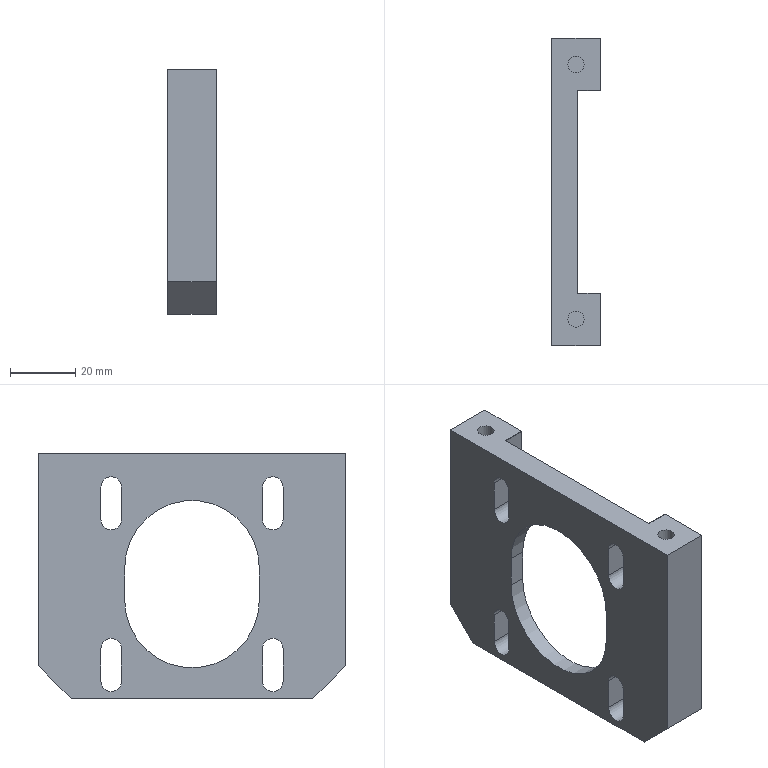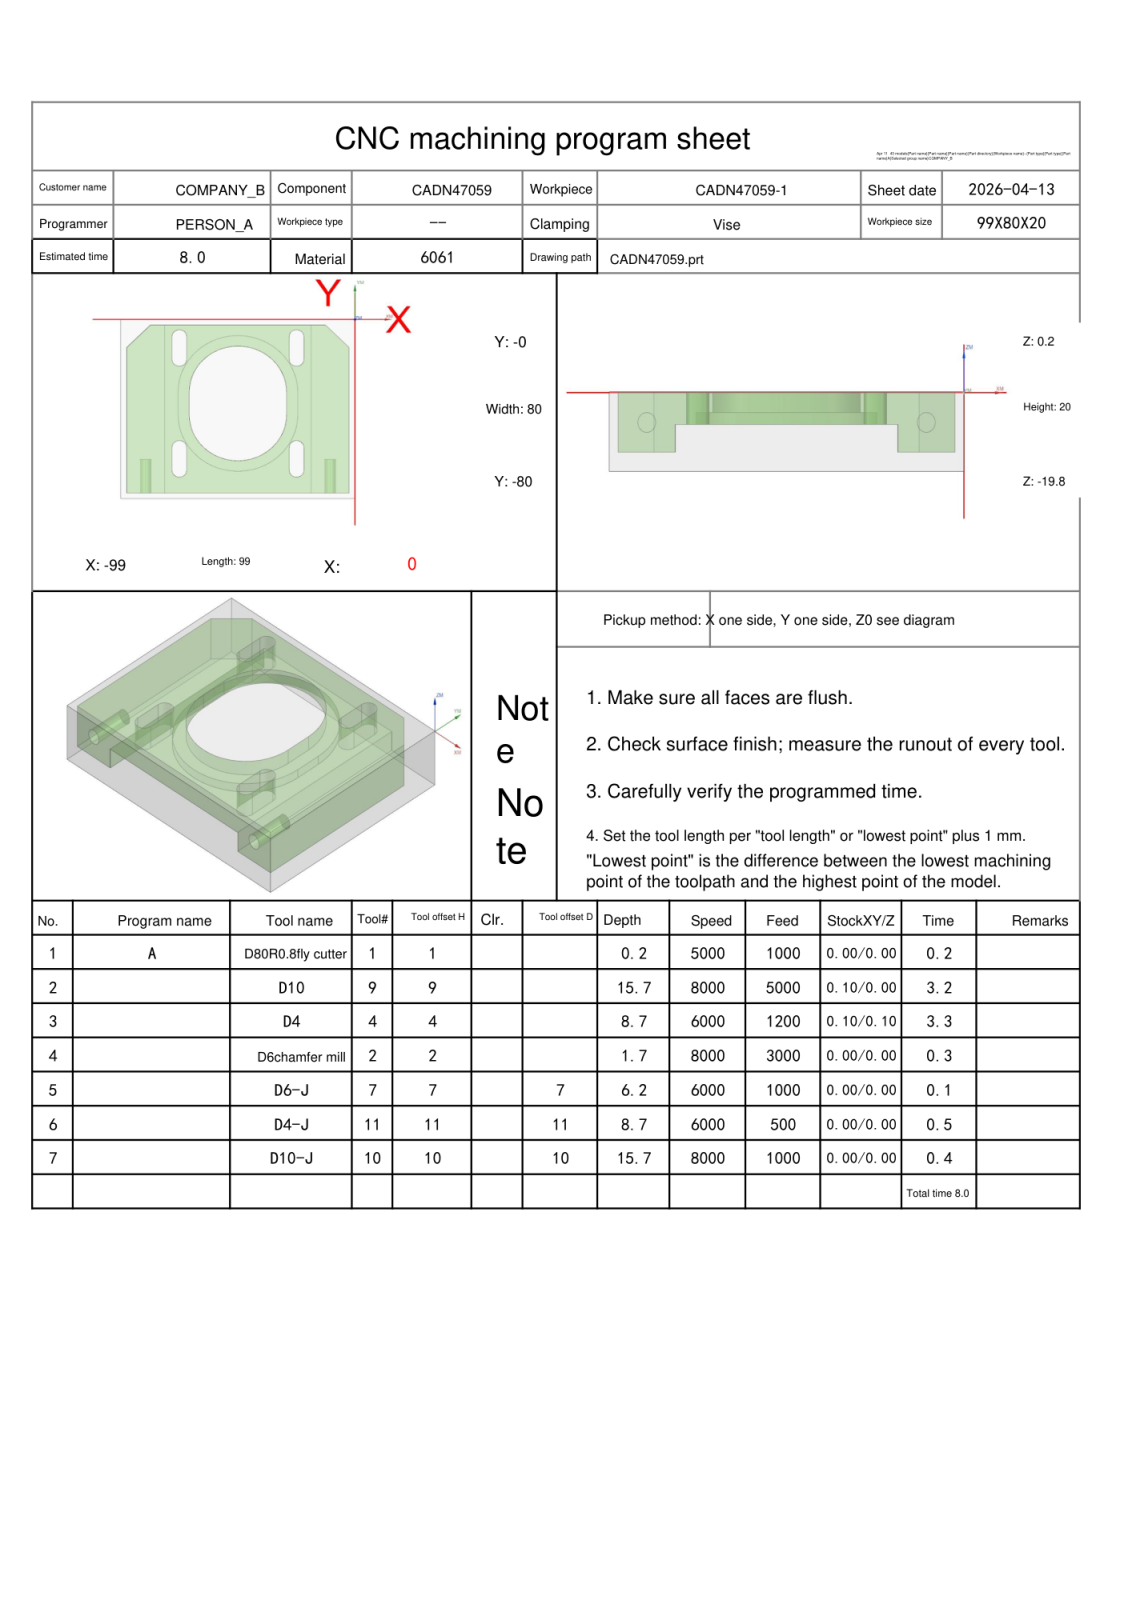NC program | NX | posted by the shop | part box 15 x 94 x 75 mm
Lines 938 to 2209 of 2209, first 1198 of 1272 lines:
N3 T04 M06
(D4  D=4. R=0. H=04 ce=0.10 di=0.10)
G00 G90 G54 X-25.801 Y-62.249 M03 S6000
G43 H04 Z20.
M08
Z.5
G01 Y-67.249 Z.453 F1200.
G03 X-24.751 Y-68.299 Z.438 I1.05 J0.0
X-23.701 Y-67.249 Z.422 I0.0 J1.05
G01 Y-57.249 Z.328
G03 X-24.751 Y-56.199 Z.313 I-1.05 J0.0
X-25.801 Y-57.249 Z.297 I0.0 J-1.05
G01 Y-67.249 Z.203
G03 X-24.751 Y-68.299 Z.188 I1.05 J0.0
X-23.701 Y-67.249 Z.172 I0.0 J1.05
G01 Y-57.249 Z.078
G03 X-24.751 Y-56.199 Z.063 I-1.05 J0.0
X-25.801 Y-57.249 Z.047 I0.0 J-1.05
G01 Y-67.249 Z-.047
G03 X-24.751 Y-68.299 Z-.063 I1.05 J0.0
X-23.701 Y-67.249 Z-.078 I0.0 J1.05
G01 Y-57.249 Z-.172
G03 X-24.751 Y-56.199 Z-.188 I-1.05 J0.0
X-25.801 Y-57.249 Z-.203 I0.0 J-1.05
G01 Y-67.249 Z-.297
G03 X-24.751 Y-68.299 Z-.313 I1.05 J0.0
X-23.701 Y-67.249 Z-.328 I0.0 J1.05
G01 Y-57.249 Z-.422
G03 X-24.751 Y-56.199 Z-.438 I-1.05 J0.0
X-25.801 Y-57.249 Z-.453 I0.0 J-1.05
G01 Y-67.249 Z-.547
G03 X-24.751 Y-68.299 Z-.563 I1.05 J0.0
X-23.701 Y-67.249 Z-.578 I0.0 J1.05
G01 Y-57.249 Z-.672
G03 X-24.751 Y-56.199 Z-.688 I-1.05 J0.0
X-25.801 Y-57.249 Z-.703 I0.0 J-1.05
G01 Y-67.249 Z-.797
G03 X-24.751 Y-68.299 Z-.813 I1.05 J0.0
X-23.701 Y-67.249 Z-.828 I0.0 J1.05
G01 Y-57.249 Z-.922
G03 X-24.751 Y-56.199 Z-.938 I-1.05 J0.0
X-25.801 Y-57.249 Z-.953 I0.0 J-1.05
G01 Y-67.249 Z-1.047
G03 X-24.751 Y-68.299 Z-1.063 I1.05 J0.0
X-23.701 Y-67.249 Z-1.078 I0.0 J1.05
G01 Y-57.249 Z-1.172
G03 X-24.751 Y-56.199 Z-1.188 I-1.05 J0.0
X-25.801 Y-57.249 Z-1.203 I0.0 J-1.05
G01 Y-67.249 Z-1.297
G03 X-24.751 Y-68.299 Z-1.313 I1.05 J0.0
X-23.701 Y-67.249 Z-1.328 I0.0 J1.05
G01 Y-57.249 Z-1.422
G03 X-24.751 Y-56.199 Z-1.438 I-1.05 J0.0
X-25.801 Y-57.249 Z-1.453 I0.0 J-1.05
G01 Y-67.249 Z-1.547
G03 X-24.751 Y-68.299 Z-1.563 I1.05 J0.0
X-23.701 Y-67.249 Z-1.578 I0.0 J1.05
G01 Y-57.249 Z-1.672
G03 X-24.751 Y-56.199 Z-1.688 I-1.05 J0.0
X-25.801 Y-57.249 Z-1.703 I0.0 J-1.05
G01 Y-67.249 Z-1.797
G03 X-24.751 Y-68.299 Z-1.813 I1.05 J0.0
X-23.701 Y-67.249 Z-1.828 I0.0 J1.05
G01 Y-57.249 Z-1.922
G03 X-24.751 Y-56.199 Z-1.938 I-1.05 J0.0
X-25.801 Y-57.249 Z-1.953 I0.0 J-1.05
G01 Y-67.249 Z-2.047
G03 X-24.751 Y-68.299 Z-2.063 I1.05 J0.0
X-23.701 Y-67.249 Z-2.078 I0.0 J1.05
G01 Y-57.249 Z-2.172
G03 X-24.751 Y-56.199 Z-2.188 I-1.05 J0.0
X-25.801 Y-57.249 Z-2.203 I0.0 J-1.05
G01 Y-67.249 Z-2.297
G03 X-24.751 Y-68.299 Z-2.313 I1.05 J0.0
X-23.701 Y-67.249 Z-2.328 I0.0 J1.05
G01 Y-57.249 Z-2.422
G03 X-24.751 Y-56.199 Z-2.438 I-1.05 J0.0
X-25.801 Y-57.249 Z-2.453 I0.0 J-1.05
G01 Y-67.249 Z-2.547
G03 X-24.751 Y-68.299 Z-2.563 I1.05 J0.0
X-23.701 Y-67.249 Z-2.578 I0.0 J1.05
G01 Y-57.249 Z-2.672
G03 X-24.751 Y-56.199 Z-2.688 I-1.05 J0.0
X-25.801 Y-57.249 Z-2.703 I0.0 J-1.05
G01 Y-67.249 Z-2.797
G03 X-24.751 Y-68.299 Z-2.813 I1.05 J0.0
X-23.701 Y-67.249 Z-2.828 I0.0 J1.05
G01 Y-57.249 Z-2.922
G03 X-24.751 Y-56.199 Z-2.938 I-1.05 J0.0
X-25.801 Y-57.249 Z-2.953 I0.0 J-1.05
G01 Y-67.249 Z-3.047
G03 X-24.751 Y-68.299 Z-3.063 I1.05 J0.0
X-23.701 Y-67.249 Z-3.078 I0.0 J1.05
G01 Y-57.249 Z-3.172
G03 X-24.751 Y-56.199 Z-3.188 I-1.05 J0.0
X-25.801 Y-57.249 Z-3.203 I0.0 J-1.05
G01 Y-67.249 Z-3.297
G03 X-24.751 Y-68.299 Z-3.313 I1.05 J0.0
X-23.701 Y-67.249 Z-3.328 I0.0 J1.05
G01 Y-57.249 Z-3.422
G03 X-24.751 Y-56.199 Z-3.438 I-1.05 J0.0
X-25.801 Y-57.249 Z-3.453 I0.0 J-1.05
G01 Y-67.249 Z-3.547
G03 X-24.751 Y-68.299 Z-3.563 I1.05 J0.0
X-23.701 Y-67.249 Z-3.578 I0.0 J1.05
G01 Y-57.249 Z-3.672
G03 X-24.751 Y-56.199 Z-3.688 I-1.05 J0.0
X-25.801 Y-57.249 Z-3.703 I0.0 J-1.05
G01 Y-67.249 Z-3.797
G03 X-24.751 Y-68.299 Z-3.813 I1.05 J0.0
X-23.701 Y-67.249 Z-3.828 I0.0 J1.05
G01 Y-57.249 Z-3.922
G03 X-24.751 Y-56.199 Z-3.938 I-1.05 J0.0
X-25.801 Y-57.249 Z-3.953 I0.0 J-1.05
G01 Y-67.249 Z-4.047
G03 X-24.751 Y-68.299 Z-4.063 I1.05 J0.0
X-23.701 Y-67.249 Z-4.078 I0.0 J1.05
G01 Y-57.249 Z-4.172
G03 X-24.751 Y-56.199 Z-4.188 I-1.05 J0.0
X-25.801 Y-57.249 Z-4.203 I0.0 J-1.05
G01 Y-67.249 Z-4.297
G03 X-24.751 Y-68.299 Z-4.313 I1.05 J0.0
X-23.701 Y-67.249 Z-4.328 I0.0 J1.05
G01 Y-57.249 Z-4.422
G03 X-24.751 Y-56.199 Z-4.438 I-1.05 J0.0
X-25.801 Y-57.249 Z-4.453 I0.0 J-1.05
G01 Y-67.249 Z-4.547
G03 X-24.751 Y-68.299 Z-4.563 I1.05 J0.0
X-23.701 Y-67.249 Z-4.578 I0.0 J1.05
G01 Y-57.249 Z-4.672
G03 X-24.751 Y-56.199 Z-4.688 I-1.05 J0.0
X-25.801 Y-57.249 Z-4.703 I0.0 J-1.05
G01 Y-67.249 Z-4.797
G03 X-24.751 Y-68.299 Z-4.813 I1.05 J0.0
X-23.701 Y-67.249 Z-4.828 I0.0 J1.05
G01 Y-57.249 Z-4.922
G03 X-24.751 Y-56.199 Z-4.938 I-1.05 J0.0
X-25.801 Y-57.249 Z-4.953 I0.0 J-1.05
G01 Y-67.249 Z-5.047
G03 X-24.751 Y-68.299 Z-5.063 I1.05 J0.0
X-23.701 Y-67.249 Z-5.078 I0.0 J1.05
G01 Y-57.249 Z-5.172
G03 X-24.751 Y-56.199 Z-5.188 I-1.05 J0.0
X-25.801 Y-57.249 Z-5.203 I0.0 J-1.05
G01 Y-67.249 Z-5.297
G03 X-24.751 Y-68.299 Z-5.313 I1.05 J0.0
X-23.701 Y-67.249 Z-5.328 I0.0 J1.05
G01 Y-57.249 Z-5.422
G03 X-24.751 Y-56.199 Z-5.438 I-1.05 J0.0
X-25.801 Y-57.249 Z-5.453 I0.0 J-1.05
G01 Y-67.249 Z-5.547
G03 X-24.751 Y-68.299 Z-5.563 I1.05 J0.0
X-23.701 Y-67.249 Z-5.578 I0.0 J1.05
G01 Y-57.249 Z-5.672
G03 X-24.751 Y-56.199 Z-5.688 I-1.05 J0.0
X-25.801 Y-57.249 Z-5.703 I0.0 J-1.05
G01 Y-67.249 Z-5.797
G03 X-24.751 Y-68.299 Z-5.813 I1.05 J0.0
X-23.701 Y-67.249 Z-5.828 I0.0 J1.05
G01 Y-57.249 Z-5.922
G03 X-24.751 Y-56.199 Z-5.938 I-1.05 J0.0
X-25.801 Y-57.249 Z-5.953 I0.0 J-1.05
G01 Y-67.249 Z-6.047
G03 X-24.751 Y-68.299 Z-6.063 I1.05 J0.0
X-23.701 Y-67.249 Z-6.078 I0.0 J1.05
G01 Y-57.249 Z-6.172
G03 X-24.751 Y-56.199 Z-6.188 I-1.05 J0.0
X-25.801 Y-57.249 Z-6.203 I0.0 J-1.05
G01 Y-67.249 Z-6.297
G03 X-24.751 Y-68.299 Z-6.313 I1.05 J0.0
X-23.701 Y-67.249 Z-6.328 I0.0 J1.05
G01 Y-57.249 Z-6.422
G03 X-24.751 Y-56.199 Z-6.438 I-1.05 J0.0
X-25.801 Y-57.249 Z-6.453 I0.0 J-1.05
G01 Y-67.249 Z-6.547
G03 X-24.751 Y-68.299 Z-6.563 I1.05 J0.0
X-23.701 Y-67.249 Z-6.578 I0.0 J1.05
G01 Y-57.249 Z-6.672
G03 X-24.751 Y-56.199 Z-6.688 I-1.05 J0.0
X-25.801 Y-57.249 Z-6.703 I0.0 J-1.05
G01 Y-67.249 Z-6.797
G03 X-24.751 Y-68.299 Z-6.813 I1.05 J0.0
X-23.701 Y-67.249 Z-6.828 I0.0 J1.05
G01 Y-57.249 Z-6.922
G03 X-24.751 Y-56.199 Z-6.938 I-1.05 J0.0
X-25.801 Y-57.249 Z-6.953 I0.0 J-1.05
G01 Y-67.249 Z-7.047
G03 X-24.751 Y-68.299 Z-7.063 I1.05 J0.0
X-23.701 Y-67.249 Z-7.078 I0.0 J1.05
G01 Y-57.249 Z-7.172
G03 X-24.751 Y-56.199 Z-7.188 I-1.05 J0.0
X-25.801 Y-57.249 Z-7.203 I0.0 J-1.05
G01 Y-67.249 Z-7.297
G03 X-24.751 Y-68.299 Z-7.313 I1.05 J0.0
X-23.701 Y-67.249 Z-7.328 I0.0 J1.05
G01 Y-57.249 Z-7.422
G03 X-24.751 Y-56.199 Z-7.438 I-1.05 J0.0
X-25.801 Y-57.249 Z-7.453 I0.0 J-1.05
G01 Y-67.249 Z-7.547
G03 X-24.751 Y-68.299 Z-7.563 I1.05 J0.0
X-23.701 Y-67.249 Z-7.578 I0.0 J1.05
G01 Y-57.249 Z-7.672
G03 X-24.751 Y-56.199 Z-7.688 I-1.05 J0.0
X-25.801 Y-57.249 Z-7.703 I0.0 J-1.05
G01 Y-67.249 Z-7.797
G03 X-24.751 Y-68.299 Z-7.813 I1.05 J0.0
X-23.701 Y-67.249 Z-7.828 I0.0 J1.05
G01 Y-57.249 Z-7.922
G03 X-24.751 Y-56.199 Z-7.938 I-1.05 J0.0
X-25.801 Y-57.249 Z-7.953 I0.0 J-1.05
G01 Y-67.249 Z-8.047
G03 X-24.751 Y-68.299 Z-8.063 I1.05 J0.0
X-23.701 Y-67.249 Z-8.078 I0.0 J1.05
G01 Y-57.249 Z-8.172
G03 X-24.751 Y-56.199 Z-8.188 I-1.05 J0.0
X-25.801 Y-57.249 Z-8.203 I0.0 J-1.05
G01 Y-67.249 Z-8.297
G03 X-24.751 Y-68.299 Z-8.313 I1.05 J0.0
X-23.701 Y-67.249 Z-8.328 I0.0 J1.05
G01 Y-57.249 Z-8.422
G03 X-24.751 Y-56.199 Z-8.438 I-1.05 J0.0
X-25.801 Y-57.249 Z-8.453 I0.0 J-1.05
G01 Y-62.249 Z-8.5
Y-67.249
G03 X-24.751 Y-68.299 I1.05 J0.0
X-23.701 Y-67.249 I0.0 J1.05
G01 Y-57.249
G03 X-24.751 Y-56.199 I-1.05 J0.0
X-25.801 Y-57.249 I0.0 J-1.05
G01 Y-62.249
Y-62.749
Z-7.5
G00 Z20.
X-23.701 Y-12.751
Z.5
G01 Y-7.751 Z.453
G03 X-24.751 Y-6.701 Z.438 I-1.05 J0.0
X-25.801 Y-7.751 Z.422 I0.0 J-1.05
G01 Y-17.751 Z.328
G03 X-24.751 Y-18.801 Z.313 I1.05 J0.0
X-23.701 Y-17.751 Z.297 I0.0 J1.05
G01 Y-7.751 Z.203
G03 X-24.751 Y-6.701 Z.188 I-1.05 J0.0
X-25.801 Y-7.751 Z.172 I0.0 J-1.05
G01 Y-17.751 Z.078
G03 X-24.751 Y-18.801 Z.063 I1.05 J0.0
X-23.701 Y-17.751 Z.047 I0.0 J1.05
G01 Y-7.751 Z-.047
G03 X-24.751 Y-6.701 Z-.063 I-1.05 J0.0
X-25.801 Y-7.751 Z-.078 I0.0 J-1.05
G01 Y-17.751 Z-.172
G03 X-24.751 Y-18.801 Z-.188 I1.05 J0.0
X-23.701 Y-17.751 Z-.203 I0.0 J1.05
G01 Y-7.751 Z-.297
G03 X-24.751 Y-6.701 Z-.313 I-1.05 J0.0
X-25.801 Y-7.751 Z-.328 I0.0 J-1.05
G01 Y-17.751 Z-.422
G03 X-24.751 Y-18.801 Z-.438 I1.05 J0.0
X-23.701 Y-17.751 Z-.453 I0.0 J1.05
G01 Y-7.751 Z-.547
G03 X-24.751 Y-6.701 Z-.563 I-1.05 J0.0
X-25.801 Y-7.751 Z-.578 I0.0 J-1.05
G01 Y-17.751 Z-.672
G03 X-24.751 Y-18.801 Z-.688 I1.05 J0.0
X-23.701 Y-17.751 Z-.703 I0.0 J1.05
G01 Y-7.751 Z-.797
G03 X-24.751 Y-6.701 Z-.813 I-1.05 J0.0
X-25.801 Y-7.751 Z-.828 I0.0 J-1.05
G01 Y-17.751 Z-.922
G03 X-24.751 Y-18.801 Z-.938 I1.05 J0.0
X-23.701 Y-17.751 Z-.953 I0.0 J1.05
G01 Y-7.751 Z-1.047
G03 X-24.751 Y-6.701 Z-1.063 I-1.05 J0.0
X-25.801 Y-7.751 Z-1.078 I0.0 J-1.05
G01 Y-17.751 Z-1.172
G03 X-24.751 Y-18.801 Z-1.188 I1.05 J0.0
X-23.701 Y-17.751 Z-1.203 I0.0 J1.05
G01 Y-7.751 Z-1.297
G03 X-24.751 Y-6.701 Z-1.313 I-1.05 J0.0
X-25.801 Y-7.751 Z-1.328 I0.0 J-1.05
G01 Y-17.751 Z-1.422
G03 X-24.751 Y-18.801 Z-1.438 I1.05 J0.0
X-23.701 Y-17.751 Z-1.453 I0.0 J1.05
G01 Y-7.751 Z-1.547
G03 X-24.751 Y-6.701 Z-1.563 I-1.05 J0.0
X-25.801 Y-7.751 Z-1.578 I0.0 J-1.05
G01 Y-17.751 Z-1.672
G03 X-24.751 Y-18.801 Z-1.688 I1.05 J0.0
X-23.701 Y-17.751 Z-1.703 I0.0 J1.05
G01 Y-7.751 Z-1.797
G03 X-24.751 Y-6.701 Z-1.813 I-1.05 J0.0
X-25.801 Y-7.751 Z-1.828 I0.0 J-1.05
G01 Y-17.751 Z-1.922
G03 X-24.751 Y-18.801 Z-1.938 I1.05 J0.0
X-23.701 Y-17.751 Z-1.953 I0.0 J1.05
G01 Y-7.751 Z-2.047
G03 X-24.751 Y-6.701 Z-2.063 I-1.05 J0.0
X-25.801 Y-7.751 Z-2.078 I0.0 J-1.05
G01 Y-17.751 Z-2.172
G03 X-24.751 Y-18.801 Z-2.188 I1.05 J0.0
X-23.701 Y-17.751 Z-2.203 I0.0 J1.05
G01 Y-7.751 Z-2.297
G03 X-24.751 Y-6.701 Z-2.313 I-1.05 J0.0
X-25.801 Y-7.751 Z-2.328 I0.0 J-1.05
G01 Y-17.751 Z-2.422
G03 X-24.751 Y-18.801 Z-2.438 I1.05 J0.0
X-23.701 Y-17.751 Z-2.453 I0.0 J1.05
G01 Y-7.751 Z-2.547
G03 X-24.751 Y-6.701 Z-2.563 I-1.05 J0.0
X-25.801 Y-7.751 Z-2.578 I0.0 J-1.05
G01 Y-17.751 Z-2.672
G03 X-24.751 Y-18.801 Z-2.688 I1.05 J0.0
X-23.701 Y-17.751 Z-2.703 I0.0 J1.05
G01 Y-7.751 Z-2.797
G03 X-24.751 Y-6.701 Z-2.813 I-1.05 J0.0
X-25.801 Y-7.751 Z-2.828 I0.0 J-1.05
G01 Y-17.751 Z-2.922
G03 X-24.751 Y-18.801 Z-2.938 I1.05 J0.0
X-23.701 Y-17.751 Z-2.953 I0.0 J1.05
G01 Y-7.751 Z-3.047
G03 X-24.751 Y-6.701 Z-3.063 I-1.05 J0.0
X-25.801 Y-7.751 Z-3.078 I0.0 J-1.05
G01 Y-17.751 Z-3.172
G03 X-24.751 Y-18.801 Z-3.188 I1.05 J0.0
X-23.701 Y-17.751 Z-3.203 I0.0 J1.05
G01 Y-7.751 Z-3.297
G03 X-24.751 Y-6.701 Z-3.313 I-1.05 J0.0
X-25.801 Y-7.751 Z-3.328 I0.0 J-1.05
G01 Y-17.751 Z-3.422
G03 X-24.751 Y-18.801 Z-3.438 I1.05 J0.0
X-23.701 Y-17.751 Z-3.453 I0.0 J1.05
G01 Y-7.751 Z-3.547
G03 X-24.751 Y-6.701 Z-3.563 I-1.05 J0.0
X-25.801 Y-7.751 Z-3.578 I0.0 J-1.05
G01 Y-17.751 Z-3.672
G03 X-24.751 Y-18.801 Z-3.688 I1.05 J0.0
X-23.701 Y-17.751 Z-3.703 I0.0 J1.05
G01 Y-7.751 Z-3.797
G03 X-24.751 Y-6.701 Z-3.813 I-1.05 J0.0
X-25.801 Y-7.751 Z-3.828 I0.0 J-1.05
G01 Y-17.751 Z-3.922
G03 X-24.751 Y-18.801 Z-3.938 I1.05 J0.0
X-23.701 Y-17.751 Z-3.953 I0.0 J1.05
G01 Y-7.751 Z-4.047
G03 X-24.751 Y-6.701 Z-4.063 I-1.05 J0.0
X-25.801 Y-7.751 Z-4.078 I0.0 J-1.05
G01 Y-17.751 Z-4.172
G03 X-24.751 Y-18.801 Z-4.188 I1.05 J0.0
X-23.701 Y-17.751 Z-4.203 I0.0 J1.05
G01 Y-7.751 Z-4.297
G03 X-24.751 Y-6.701 Z-4.313 I-1.05 J0.0
X-25.801 Y-7.751 Z-4.328 I0.0 J-1.05
G01 Y-17.751 Z-4.422
G03 X-24.751 Y-18.801 Z-4.438 I1.05 J0.0
X-23.701 Y-17.751 Z-4.453 I0.0 J1.05
G01 Y-7.751 Z-4.547
G03 X-24.751 Y-6.701 Z-4.563 I-1.05 J0.0
X-25.801 Y-7.751 Z-4.578 I0.0 J-1.05
G01 Y-17.751 Z-4.672
G03 X-24.751 Y-18.801 Z-4.688 I1.05 J0.0
X-23.701 Y-17.751 Z-4.703 I0.0 J1.05
G01 Y-7.751 Z-4.797
G03 X-24.751 Y-6.701 Z-4.813 I-1.05 J0.0
X-25.801 Y-7.751 Z-4.828 I0.0 J-1.05
G01 Y-17.751 Z-4.922
G03 X-24.751 Y-18.801 Z-4.938 I1.05 J0.0
X-23.701 Y-17.751 Z-4.953 I0.0 J1.05
G01 Y-7.751 Z-5.047
G03 X-24.751 Y-6.701 Z-5.063 I-1.05 J0.0
X-25.801 Y-7.751 Z-5.078 I0.0 J-1.05
G01 Y-17.751 Z-5.172
G03 X-24.751 Y-18.801 Z-5.188 I1.05 J0.0
X-23.701 Y-17.751 Z-5.203 I0.0 J1.05
G01 Y-7.751 Z-5.297
G03 X-24.751 Y-6.701 Z-5.313 I-1.05 J0.0
X-25.801 Y-7.751 Z-5.328 I0.0 J-1.05
G01 Y-17.751 Z-5.422
G03 X-24.751 Y-18.801 Z-5.438 I1.05 J0.0
X-23.701 Y-17.751 Z-5.453 I0.0 J1.05
G01 Y-7.751 Z-5.547
G03 X-24.751 Y-6.701 Z-5.563 I-1.05 J0.0
X-25.801 Y-7.751 Z-5.578 I0.0 J-1.05
G01 Y-17.751 Z-5.672
G03 X-24.751 Y-18.801 Z-5.688 I1.05 J0.0
X-23.701 Y-17.751 Z-5.703 I0.0 J1.05
G01 Y-7.751 Z-5.797
G03 X-24.751 Y-6.701 Z-5.813 I-1.05 J0.0
X-25.801 Y-7.751 Z-5.828 I0.0 J-1.05
G01 Y-17.751 Z-5.922
G03 X-24.751 Y-18.801 Z-5.938 I1.05 J0.0
X-23.701 Y-17.751 Z-5.953 I0.0 J1.05
G01 Y-7.751 Z-6.047
G03 X-24.751 Y-6.701 Z-6.063 I-1.05 J0.0
X-25.801 Y-7.751 Z-6.078 I0.0 J-1.05
G01 Y-17.751 Z-6.172
G03 X-24.751 Y-18.801 Z-6.188 I1.05 J0.0
X-23.701 Y-17.751 Z-6.203 I0.0 J1.05
G01 Y-7.751 Z-6.297
G03 X-24.751 Y-6.701 Z-6.313 I-1.05 J0.0
X-25.801 Y-7.751 Z-6.328 I0.0 J-1.05
G01 Y-17.751 Z-6.422
G03 X-24.751 Y-18.801 Z-6.438 I1.05 J0.0
X-23.701 Y-17.751 Z-6.453 I0.0 J1.05
G01 Y-7.751 Z-6.547
G03 X-24.751 Y-6.701 Z-6.563 I-1.05 J0.0
X-25.801 Y-7.751 Z-6.578 I0.0 J-1.05
G01 Y-17.751 Z-6.672
G03 X-24.751 Y-18.801 Z-6.688 I1.05 J0.0
X-23.701 Y-17.751 Z-6.703 I0.0 J1.05
G01 Y-7.751 Z-6.797
G03 X-24.751 Y-6.701 Z-6.813 I-1.05 J0.0
X-25.801 Y-7.751 Z-6.828 I0.0 J-1.05
G01 Y-17.751 Z-6.922
G03 X-24.751 Y-18.801 Z-6.938 I1.05 J0.0
X-23.701 Y-17.751 Z-6.953 I0.0 J1.05
G01 Y-7.751 Z-7.047
G03 X-24.751 Y-6.701 Z-7.063 I-1.05 J0.0
X-25.801 Y-7.751 Z-7.078 I0.0 J-1.05
G01 Y-17.751 Z-7.172
G03 X-24.751 Y-18.801 Z-7.188 I1.05 J0.0
X-23.701 Y-17.751 Z-7.203 I0.0 J1.05
G01 Y-7.751 Z-7.297
G03 X-24.751 Y-6.701 Z-7.313 I-1.05 J0.0
X-25.801 Y-7.751 Z-7.328 I0.0 J-1.05
G01 Y-17.751 Z-7.422
G03 X-24.751 Y-18.801 Z-7.438 I1.05 J0.0
X-23.701 Y-17.751 Z-7.453 I0.0 J1.05
G01 Y-7.751 Z-7.547
G03 X-24.751 Y-6.701 Z-7.563 I-1.05 J0.0
X-25.801 Y-7.751 Z-7.578 I0.0 J-1.05
G01 Y-17.751 Z-7.672
G03 X-24.751 Y-18.801 Z-7.688 I1.05 J0.0
X-23.701 Y-17.751 Z-7.703 I0.0 J1.05
G01 Y-7.751 Z-7.797
G03 X-24.751 Y-6.701 Z-7.813 I-1.05 J0.0
X-25.801 Y-7.751 Z-7.828 I0.0 J-1.05
G01 Y-17.751 Z-7.922
G03 X-24.751 Y-18.801 Z-7.938 I1.05 J0.0
X-23.701 Y-17.751 Z-7.953 I0.0 J1.05
G01 Y-7.751 Z-8.047
G03 X-24.751 Y-6.701 Z-8.063 I-1.05 J0.0
X-25.801 Y-7.751 Z-8.078 I0.0 J-1.05
G01 Y-17.751 Z-8.172
G03 X-24.751 Y-18.801 Z-8.188 I1.05 J0.0
X-23.701 Y-17.751 Z-8.203 I0.0 J1.05
G01 Y-7.751 Z-8.297
G03 X-24.751 Y-6.701 Z-8.313 I-1.05 J0.0
X-25.801 Y-7.751 Z-8.328 I0.0 J-1.05
G01 Y-17.751 Z-8.422
G03 X-24.751 Y-18.801 Z-8.438 I1.05 J0.0
X-23.701 Y-17.751 Z-8.453 I0.0 J1.05
G01 Y-12.751 Z-8.5
Y-7.751
G03 X-24.751 Y-6.701 I-1.05 J0.0
X-25.801 Y-7.751 I0.0 J-1.05
G01 Y-17.751
G03 X-24.751 Y-18.801 I1.05 J0.0
X-23.701 Y-17.751 I0.0 J1.05
G01 Y-12.751
Y-12.251
Z-7.5
G00 Z20.
X-73.199 Y-12.751
Z.5
G01 Y-7.751 Z.453
G03 X-74.249 Y-6.701 Z.438 I-1.05 J0.0
X-75.299 Y-7.751 Z.422 I0.0 J-1.05
G01 Y-17.751 Z.328
G03 X-74.249 Y-18.801 Z.313 I1.05 J0.0
X-73.199 Y-17.751 Z.297 I0.0 J1.05
G01 Y-7.751 Z.203
G03 X-74.249 Y-6.701 Z.188 I-1.05 J0.0
X-75.299 Y-7.751 Z.172 I0.0 J-1.05
G01 Y-17.751 Z.078
G03 X-74.249 Y-18.801 Z.063 I1.05 J0.0
X-73.199 Y-17.751 Z.047 I0.0 J1.05
G01 Y-7.751 Z-.047
G03 X-74.249 Y-6.701 Z-.063 I-1.05 J0.0
X-75.299 Y-7.751 Z-.078 I0.0 J-1.05
G01 Y-17.751 Z-.172
G03 X-74.249 Y-18.801 Z-.188 I1.05 J0.0
X-73.199 Y-17.751 Z-.203 I0.0 J1.05
G01 Y-7.751 Z-.297
G03 X-74.249 Y-6.701 Z-.313 I-1.05 J0.0
X-75.299 Y-7.751 Z-.328 I0.0 J-1.05
G01 Y-17.751 Z-.422
G03 X-74.249 Y-18.801 Z-.438 I1.05 J0.0
X-73.199 Y-17.751 Z-.453 I0.0 J1.05
G01 Y-7.751 Z-.547
G03 X-74.249 Y-6.701 Z-.563 I-1.05 J0.0
X-75.299 Y-7.751 Z-.578 I0.0 J-1.05
G01 Y-17.751 Z-.672
G03 X-74.249 Y-18.801 Z-.688 I1.05 J0.0
X-73.199 Y-17.751 Z-.703 I0.0 J1.05
G01 Y-7.751 Z-.797
G03 X-74.249 Y-6.701 Z-.813 I-1.05 J0.0
X-75.299 Y-7.751 Z-.828 I0.0 J-1.05
G01 Y-17.751 Z-.922
G03 X-74.249 Y-18.801 Z-.938 I1.05 J0.0
X-73.199 Y-17.751 Z-.953 I0.0 J1.05
G01 Y-7.751 Z-1.047
G03 X-74.249 Y-6.701 Z-1.063 I-1.05 J0.0
X-75.299 Y-7.751 Z-1.078 I0.0 J-1.05
G01 Y-17.751 Z-1.172
G03 X-74.249 Y-18.801 Z-1.188 I1.05 J0.0
X-73.199 Y-17.751 Z-1.203 I0.0 J1.05
G01 Y-7.751 Z-1.297
G03 X-74.249 Y-6.701 Z-1.313 I-1.05 J0.0
X-75.299 Y-7.751 Z-1.328 I0.0 J-1.05
G01 Y-17.751 Z-1.422
G03 X-74.249 Y-18.801 Z-1.438 I1.05 J0.0
X-73.199 Y-17.751 Z-1.453 I0.0 J1.05
G01 Y-7.751 Z-1.547
G03 X-74.249 Y-6.701 Z-1.563 I-1.05 J0.0
X-75.299 Y-7.751 Z-1.578 I0.0 J-1.05
G01 Y-17.751 Z-1.672
G03 X-74.249 Y-18.801 Z-1.688 I1.05 J0.0
X-73.199 Y-17.751 Z-1.703 I0.0 J1.05
G01 Y-7.751 Z-1.797
G03 X-74.249 Y-6.701 Z-1.813 I-1.05 J0.0
X-75.299 Y-7.751 Z-1.828 I0.0 J-1.05
G01 Y-17.751 Z-1.922
G03 X-74.249 Y-18.801 Z-1.938 I1.05 J0.0
X-73.199 Y-17.751 Z-1.953 I0.0 J1.05
G01 Y-7.751 Z-2.047
G03 X-74.249 Y-6.701 Z-2.063 I-1.05 J0.0
X-75.299 Y-7.751 Z-2.078 I0.0 J-1.05
G01 Y-17.751 Z-2.172
G03 X-74.249 Y-18.801 Z-2.188 I1.05 J0.0
X-73.199 Y-17.751 Z-2.203 I0.0 J1.05
G01 Y-7.751 Z-2.297
G03 X-74.249 Y-6.701 Z-2.313 I-1.05 J0.0
X-75.299 Y-7.751 Z-2.328 I0.0 J-1.05
G01 Y-17.751 Z-2.422
G03 X-74.249 Y-18.801 Z-2.438 I1.05 J0.0
X-73.199 Y-17.751 Z-2.453 I0.0 J1.05
G01 Y-7.751 Z-2.547
G03 X-74.249 Y-6.701 Z-2.563 I-1.05 J0.0
X-75.299 Y-7.751 Z-2.578 I0.0 J-1.05
G01 Y-17.751 Z-2.672
G03 X-74.249 Y-18.801 Z-2.688 I1.05 J0.0
X-73.199 Y-17.751 Z-2.703 I0.0 J1.05
G01 Y-7.751 Z-2.797
G03 X-74.249 Y-6.701 Z-2.813 I-1.05 J0.0
X-75.299 Y-7.751 Z-2.828 I0.0 J-1.05
G01 Y-17.751 Z-2.922
G03 X-74.249 Y-18.801 Z-2.938 I1.05 J0.0
X-73.199 Y-17.751 Z-2.953 I0.0 J1.05
G01 Y-7.751 Z-3.047
G03 X-74.249 Y-6.701 Z-3.063 I-1.05 J0.0
X-75.299 Y-7.751 Z-3.078 I0.0 J-1.05
G01 Y-17.751 Z-3.172
G03 X-74.249 Y-18.801 Z-3.188 I1.05 J0.0
X-73.199 Y-17.751 Z-3.203 I0.0 J1.05
G01 Y-7.751 Z-3.297
G03 X-74.249 Y-6.701 Z-3.313 I-1.05 J0.0
X-75.299 Y-7.751 Z-3.328 I0.0 J-1.05
G01 Y-17.751 Z-3.422
G03 X-74.249 Y-18.801 Z-3.438 I1.05 J0.0
X-73.199 Y-17.751 Z-3.453 I0.0 J1.05
G01 Y-7.751 Z-3.547
G03 X-74.249 Y-6.701 Z-3.563 I-1.05 J0.0
X-75.299 Y-7.751 Z-3.578 I0.0 J-1.05
G01 Y-17.751 Z-3.672
G03 X-74.249 Y-18.801 Z-3.688 I1.05 J0.0
X-73.199 Y-17.751 Z-3.703 I0.0 J1.05
G01 Y-7.751 Z-3.797
G03 X-74.249 Y-6.701 Z-3.813 I-1.05 J0.0
X-75.299 Y-7.751 Z-3.828 I0.0 J-1.05
G01 Y-17.751 Z-3.922
G03 X-74.249 Y-18.801 Z-3.938 I1.05 J0.0
X-73.199 Y-17.751 Z-3.953 I0.0 J1.05
G01 Y-7.751 Z-4.047
G03 X-74.249 Y-6.701 Z-4.063 I-1.05 J0.0
X-75.299 Y-7.751 Z-4.078 I0.0 J-1.05
G01 Y-17.751 Z-4.172
G03 X-74.249 Y-18.801 Z-4.188 I1.05 J0.0
X-73.199 Y-17.751 Z-4.203 I0.0 J1.05
G01 Y-7.751 Z-4.297
G03 X-74.249 Y-6.701 Z-4.313 I-1.05 J0.0
X-75.299 Y-7.751 Z-4.328 I0.0 J-1.05
G01 Y-17.751 Z-4.422
G03 X-74.249 Y-18.801 Z-4.438 I1.05 J0.0
X-73.199 Y-17.751 Z-4.453 I0.0 J1.05
G01 Y-7.751 Z-4.547
G03 X-74.249 Y-6.701 Z-4.563 I-1.05 J0.0
X-75.299 Y-7.751 Z-4.578 I0.0 J-1.05
G01 Y-17.751 Z-4.672
G03 X-74.249 Y-18.801 Z-4.688 I1.05 J0.0
X-73.199 Y-17.751 Z-4.703 I0.0 J1.05
G01 Y-7.751 Z-4.797
G03 X-74.249 Y-6.701 Z-4.813 I-1.05 J0.0
X-75.299 Y-7.751 Z-4.828 I0.0 J-1.05
G01 Y-17.751 Z-4.922
G03 X-74.249 Y-18.801 Z-4.938 I1.05 J0.0
X-73.199 Y-17.751 Z-4.953 I0.0 J1.05
G01 Y-7.751 Z-5.047
G03 X-74.249 Y-6.701 Z-5.063 I-1.05 J0.0
X-75.299 Y-7.751 Z-5.078 I0.0 J-1.05
G01 Y-17.751 Z-5.172
G03 X-74.249 Y-18.801 Z-5.188 I1.05 J0.0
X-73.199 Y-17.751 Z-5.203 I0.0 J1.05
G01 Y-7.751 Z-5.297
G03 X-74.249 Y-6.701 Z-5.313 I-1.05 J0.0
X-75.299 Y-7.751 Z-5.328 I0.0 J-1.05
G01 Y-17.751 Z-5.422
G03 X-74.249 Y-18.801 Z-5.438 I1.05 J0.0
X-73.199 Y-17.751 Z-5.453 I0.0 J1.05
G01 Y-7.751 Z-5.547
G03 X-74.249 Y-6.701 Z-5.563 I-1.05 J0.0
X-75.299 Y-7.751 Z-5.578 I0.0 J-1.05
G01 Y-17.751 Z-5.672
G03 X-74.249 Y-18.801 Z-5.688 I1.05 J0.0
X-73.199 Y-17.751 Z-5.703 I0.0 J1.05
G01 Y-7.751 Z-5.797
G03 X-74.249 Y-6.701 Z-5.813 I-1.05 J0.0
X-75.299 Y-7.751 Z-5.828 I0.0 J-1.05
G01 Y-17.751 Z-5.922
G03 X-74.249 Y-18.801 Z-5.938 I1.05 J0.0
X-73.199 Y-17.751 Z-5.953 I0.0 J1.05
G01 Y-7.751 Z-6.047
G03 X-74.249 Y-6.701 Z-6.063 I-1.05 J0.0
X-75.299 Y-7.751 Z-6.078 I0.0 J-1.05
G01 Y-17.751 Z-6.172
G03 X-74.249 Y-18.801 Z-6.188 I1.05 J0.0
X-73.199 Y-17.751 Z-6.203 I0.0 J1.05
G01 Y-7.751 Z-6.297
G03 X-74.249 Y-6.701 Z-6.313 I-1.05 J0.0
X-75.299 Y-7.751 Z-6.328 I0.0 J-1.05
G01 Y-17.751 Z-6.422
G03 X-74.249 Y-18.801 Z-6.438 I1.05 J0.0
X-73.199 Y-17.751 Z-6.453 I0.0 J1.05
G01 Y-7.751 Z-6.547
G03 X-74.249 Y-6.701 Z-6.563 I-1.05 J0.0
X-75.299 Y-7.751 Z-6.578 I0.0 J-1.05
G01 Y-17.751 Z-6.672
G03 X-74.249 Y-18.801 Z-6.688 I1.05 J0.0
X-73.199 Y-17.751 Z-6.703 I0.0 J1.05
G01 Y-7.751 Z-6.797
G03 X-74.249 Y-6.701 Z-6.813 I-1.05 J0.0
X-75.299 Y-7.751 Z-6.828 I0.0 J-1.05
G01 Y-17.751 Z-6.922
G03 X-74.249 Y-18.801 Z-6.938 I1.05 J0.0
X-73.199 Y-17.751 Z-6.953 I0.0 J1.05
G01 Y-7.751 Z-7.047
G03 X-74.249 Y-6.701 Z-7.063 I-1.05 J0.0
X-75.299 Y-7.751 Z-7.078 I0.0 J-1.05
G01 Y-17.751 Z-7.172
G03 X-74.249 Y-18.801 Z-7.188 I1.05 J0.0
X-73.199 Y-17.751 Z-7.203 I0.0 J1.05
G01 Y-7.751 Z-7.297
G03 X-74.249 Y-6.701 Z-7.313 I-1.05 J0.0
X-75.299 Y-7.751 Z-7.328 I0.0 J-1.05
G01 Y-17.751 Z-7.422
G03 X-74.249 Y-18.801 Z-7.438 I1.05 J0.0
X-73.199 Y-17.751 Z-7.453 I0.0 J1.05
G01 Y-7.751 Z-7.547
G03 X-74.249 Y-6.701 Z-7.563 I-1.05 J0.0
X-75.299 Y-7.751 Z-7.578 I0.0 J-1.05
G01 Y-17.751 Z-7.672
G03 X-74.249 Y-18.801 Z-7.688 I1.05 J0.0
X-73.199 Y-17.751 Z-7.703 I0.0 J1.05
G01 Y-7.751 Z-7.797
G03 X-74.249 Y-6.701 Z-7.813 I-1.05 J0.0
X-75.299 Y-7.751 Z-7.828 I0.0 J-1.05
G01 Y-17.751 Z-7.922
G03 X-74.249 Y-18.801 Z-7.938 I1.05 J0.0
X-73.199 Y-17.751 Z-7.953 I0.0 J1.05
G01 Y-7.751 Z-8.047
G03 X-74.249 Y-6.701 Z-8.063 I-1.05 J0.0
X-75.299 Y-7.751 Z-8.078 I0.0 J-1.05
G01 Y-17.751 Z-8.172
G03 X-74.249 Y-18.801 Z-8.188 I1.05 J0.0
X-73.199 Y-17.751 Z-8.203 I0.0 J1.05
G01 Y-7.751 Z-8.297
G03 X-74.249 Y-6.701 Z-8.313 I-1.05 J0.0
X-75.299 Y-7.751 Z-8.328 I0.0 J-1.05
G01 Y-17.751 Z-8.422
G03 X-74.249 Y-18.801 Z-8.438 I1.05 J0.0
X-73.199 Y-17.751 Z-8.453 I0.0 J1.05
G01 Y-12.751 Z-8.5
Y-7.751
G03 X-74.249 Y-6.701 I-1.05 J0.0
X-75.299 Y-7.751 I0.0 J-1.05
G01 Y-17.751
G03 X-74.249 Y-18.801 I1.05 J0.0
X-73.199 Y-17.751 I0.0 J1.05
G01 Y-12.751
Y-12.251
Z-7.5
G00 Z20.
Y-62.249
Z.5
G01 Y-57.249 Z.453
G03 X-74.249 Y-56.199 Z.438 I-1.05 J0.0
X-75.299 Y-57.249 Z.422 I0.0 J-1.05
G01 Y-67.249 Z.328
G03 X-74.249 Y-68.299 Z.313 I1.05 J0.0
X-73.199 Y-67.249 Z.297 I0.0 J1.05
G01 Y-57.249 Z.203
G03 X-74.249 Y-56.199 Z.188 I-1.05 J0.0
X-75.299 Y-57.249 Z.172 I0.0 J-1.05
G01 Y-67.249 Z.078
G03 X-74.249 Y-68.299 Z.063 I1.05 J0.0
X-73.199 Y-67.249 Z.047 I0.0 J1.05
G01 Y-57.249 Z-.047
G03 X-74.249 Y-56.199 Z-.063 I-1.05 J0.0
X-75.299 Y-57.249 Z-.078 I0.0 J-1.05
G01 Y-67.249 Z-.172
G03 X-74.249 Y-68.299 Z-.188 I1.05 J0.0
X-73.199 Y-67.249 Z-.203 I0.0 J1.05
G01 Y-57.249 Z-.297
G03 X-74.249 Y-56.199 Z-.313 I-1.05 J0.0
X-75.299 Y-57.249 Z-.328 I0.0 J-1.05
G01 Y-67.249 Z-.422
G03 X-74.249 Y-68.299 Z-.438 I1.05 J0.0
X-73.199 Y-67.249 Z-.453 I0.0 J1.05
G01 Y-57.249 Z-.547
G03 X-74.249 Y-56.199 Z-.563 I-1.05 J0.0
X-75.299 Y-57.249 Z-.578 I0.0 J-1.05
G01 Y-67.249 Z-.672
G03 X-74.249 Y-68.299 Z-.688 I1.05 J0.0
X-73.199 Y-67.249 Z-.703 I0.0 J1.05
G01 Y-57.249 Z-.797
G03 X-74.249 Y-56.199 Z-.813 I-1.05 J0.0
X-75.299 Y-57.249 Z-.828 I0.0 J-1.05
G01 Y-67.249 Z-.922
G03 X-74.249 Y-68.299 Z-.938 I1.05 J0.0
X-73.199 Y-67.249 Z-.953 I0.0 J1.05
G01 Y-57.249 Z-1.047
G03 X-74.249 Y-56.199 Z-1.063 I-1.05 J0.0
X-75.299 Y-57.249 Z-1.078 I0.0 J-1.05
G01 Y-67.249 Z-1.172
G03 X-74.249 Y-68.299 Z-1.188 I1.05 J0.0
X-73.199 Y-67.249 Z-1.203 I0.0 J1.05
G01 Y-57.249 Z-1.297
G03 X-74.249 Y-56.199 Z-1.313 I-1.05 J0.0
X-75.299 Y-57.249 Z-1.328 I0.0 J-1.05
G01 Y-67.249 Z-1.422
G03 X-74.249 Y-68.299 Z-1.438 I1.05 J0.0
X-73.199 Y-67.249 Z-1.453 I0.0 J1.05
G01 Y-57.249 Z-1.547
G03 X-74.249 Y-56.199 Z-1.563 I-1.05 J0.0
X-75.299 Y-57.249 Z-1.578 I0.0 J-1.05
G01 Y-67.249 Z-1.672
G03 X-74.249 Y-68.299 Z-1.688 I1.05 J0.0
X-73.199 Y-67.249 Z-1.703 I0.0 J1.05
G01 Y-57.249 Z-1.797
G03 X-74.249 Y-56.199 Z-1.813 I-1.05 J0.0
X-75.299 Y-57.249 Z-1.828 I0.0 J-1.05
G01 Y-67.249 Z-1.922
G03 X-74.249 Y-68.299 Z-1.938 I1.05 J0.0
X-73.199 Y-67.249 Z-1.953 I0.0 J1.05
G01 Y-57.249 Z-2.047
G03 X-74.249 Y-56.199 Z-2.063 I-1.05 J0.0
X-75.299 Y-57.249 Z-2.078 I0.0 J-1.05
G01 Y-67.249 Z-2.172
G03 X-74.249 Y-68.299 Z-2.188 I1.05 J0.0
X-73.199 Y-67.249 Z-2.203 I0.0 J1.05
G01 Y-57.249 Z-2.297
G03 X-74.249 Y-56.199 Z-2.313 I-1.05 J0.0
X-75.299 Y-57.249 Z-2.328 I0.0 J-1.05
G01 Y-67.249 Z-2.422
G03 X-74.249 Y-68.299 Z-2.438 I1.05 J0.0
X-73.199 Y-67.249 Z-2.453 I0.0 J1.05
G01 Y-57.249 Z-2.547
G03 X-74.249 Y-56.199 Z-2.563 I-1.05 J0.0
X-75.299 Y-57.249 Z-2.578 I0.0 J-1.05
G01 Y-67.249 Z-2.672
G03 X-74.249 Y-68.299 Z-2.688 I1.05 J0.0
X-73.199 Y-67.249 Z-2.703 I0.0 J1.05
G01 Y-57.249 Z-2.797
G03 X-74.249 Y-56.199 Z-2.813 I-1.05 J0.0
X-75.299 Y-57.249 Z-2.828 I0.0 J-1.05
G01 Y-67.249 Z-2.922
G03 X-74.249 Y-68.299 Z-2.938 I1.05 J0.0
X-73.199 Y-67.249 Z-2.953 I0.0 J1.05
G01 Y-57.249 Z-3.047
G03 X-74.249 Y-56.199 Z-3.063 I-1.05 J0.0
X-75.299 Y-57.249 Z-3.078 I0.0 J-1.05
G01 Y-67.249 Z-3.172
G03 X-74.249 Y-68.299 Z-3.188 I1.05 J0.0
X-73.199 Y-67.249 Z-3.203 I0.0 J1.05
G01 Y-57.249 Z-3.297
G03 X-74.249 Y-56.199 Z-3.313 I-1.05 J0.0
X-75.299 Y-57.249 Z-3.328 I0.0 J-1.05
G01 Y-67.249 Z-3.422
G03 X-74.249 Y-68.299 Z-3.438 I1.05 J0.0
X-73.199 Y-67.249 Z-3.453 I0.0 J1.05
G01 Y-57.249 Z-3.547
G03 X-74.249 Y-56.199 Z-3.563 I-1.05 J0.0
X-75.299 Y-57.249 Z-3.578 I0.0 J-1.05
G01 Y-67.249 Z-3.672
G03 X-74.249 Y-68.299 Z-3.688 I1.05 J0.0
X-73.199 Y-67.249 Z-3.703 I0.0 J1.05
G01 Y-57.249 Z-3.797
G03 X-74.249 Y-56.199 Z-3.813 I-1.05 J0.0
X-75.299 Y-57.249 Z-3.828 I0.0 J-1.05
G01 Y-67.249 Z-3.922
G03 X-74.249 Y-68.299 Z-3.938 I1.05 J0.0
X-73.199 Y-67.249 Z-3.953 I0.0 J1.05
G01 Y-57.249 Z-4.047
G03 X-74.249 Y-56.199 Z-4.063 I-1.05 J0.0
X-75.299 Y-57.249 Z-4.078 I0.0 J-1.05
G01 Y-67.249 Z-4.172
G03 X-74.249 Y-68.299 Z-4.188 I1.05 J0.0
X-73.199 Y-67.249 Z-4.203 I0.0 J1.05
G01 Y-57.249 Z-4.297
G03 X-74.249 Y-56.199 Z-4.313 I-1.05 J0.0
X-75.299 Y-57.249 Z-4.328 I0.0 J-1.05
G01 Y-67.249 Z-4.422
G03 X-74.249 Y-68.299 Z-4.438 I1.05 J0.0
X-73.199 Y-67.249 Z-4.453 I0.0 J1.05
G01 Y-57.249 Z-4.547
G03 X-74.249 Y-56.199 Z-4.563 I-1.05 J0.0
X-75.299 Y-57.249 Z-4.578 I0.0 J-1.05
G01 Y-67.249 Z-4.672
G03 X-74.249 Y-68.299 Z-4.688 I1.05 J0.0
X-73.199 Y-67.249 Z-4.703 I0.0 J1.05
G01 Y-57.249 Z-4.797
G03 X-74.249 Y-56.199 Z-4.813 I-1.05 J0.0
X-75.299 Y-57.249 Z-4.828 I0.0 J-1.05
G01 Y-67.249 Z-4.922
G03 X-74.249 Y-68.299 Z-4.938 I1.05 J0.0
X-73.199 Y-67.249 Z-4.953 I0.0 J1.05
G01 Y-57.249 Z-5.047
G03 X-74.249 Y-56.199 Z-5.063 I-1.05 J0.0
X-75.299 Y-57.249 Z-5.078 I0.0 J-1.05
G01 Y-67.249 Z-5.172
G03 X-74.249 Y-68.299 Z-5.188 I1.05 J0.0
X-73.199 Y-67.249 Z-5.203 I0.0 J1.05
G01 Y-57.249 Z-5.297
G03 X-74.249 Y-56.199 Z-5.313 I-1.05 J0.0
X-75.299 Y-57.249 Z-5.328 I0.0 J-1.05
G01 Y-67.249 Z-5.422
G03 X-74.249 Y-68.299 Z-5.438 I1.05 J0.0
X-73.199 Y-67.249 Z-5.453 I0.0 J1.05
G01 Y-57.249 Z-5.547
G03 X-74.249 Y-56.199 Z-5.563 I-1.05 J0.0
X-75.299 Y-57.249 Z-5.578 I0.0 J-1.05
G01 Y-67.249 Z-5.672
G03 X-74.249 Y-68.299 Z-5.688 I1.05 J0.0
X-73.199 Y-67.249 Z-5.703 I0.0 J1.05
G01 Y-57.249 Z-5.797
G03 X-74.249 Y-56.199 Z-5.813 I-1.05 J0.0
X-75.299 Y-57.249 Z-5.828 I0.0 J-1.05
G01 Y-67.249 Z-5.922
G03 X-74.249 Y-68.299 Z-5.938 I1.05 J0.0
X-73.199 Y-67.249 Z-5.953 I0.0 J1.05
G01 Y-57.249 Z-6.047
G03 X-74.249 Y-56.199 Z-6.063 I-1.05 J0.0
X-75.299 Y-57.249 Z-6.078 I0.0 J-1.05
G01 Y-67.249 Z-6.172
G03 X-74.249 Y-68.299 Z-6.188 I1.05 J0.0
X-73.199 Y-67.249 Z-6.203 I0.0 J1.05
G01 Y-57.249 Z-6.297
G03 X-74.249 Y-56.199 Z-6.313 I-1.05 J0.0
X-75.299 Y-57.249 Z-6.328 I0.0 J-1.05
G01 Y-67.249 Z-6.422
G03 X-74.249 Y-68.299 Z-6.438 I1.05 J0.0
X-73.199 Y-67.249 Z-6.453 I0.0 J1.05
G01 Y-57.249 Z-6.547
G03 X-74.249 Y-56.199 Z-6.563 I-1.05 J0.0
X-75.299 Y-57.249 Z-6.578 I0.0 J-1.05
G01 Y-67.249 Z-6.672
G03 X-74.249 Y-68.299 Z-6.688 I1.05 J0.0
X-73.199 Y-67.249 Z-6.703 I0.0 J1.05
G01 Y-57.249 Z-6.797
G03 X-74.249 Y-56.199 Z-6.813 I-1.05 J0.0
X-75.299 Y-57.249 Z-6.828 I0.0 J-1.05
G01 Y-67.249 Z-6.922
G03 X-74.249 Y-68.299 Z-6.938 I1.05 J0.0
X-73.199 Y-67.249 Z-6.953 I0.0 J1.05
G01 Y-57.249 Z-7.047
G03 X-74.249 Y-56.199 Z-7.063 I-1.05 J0.0
X-75.299 Y-57.249 Z-7.078 I0.0 J-1.05
G01 Y-67.249 Z-7.172
G03 X-74.249 Y-68.299 Z-7.188 I1.05 J0.0
X-73.199 Y-67.249 Z-7.203 I0.0 J1.05
G01 Y-57.249 Z-7.297
G03 X-74.249 Y-56.199 Z-7.313 I-1.05 J0.0
X-75.299 Y-57.249 Z-7.328 I0.0 J-1.05
G01 Y-67.249 Z-7.422
G03 X-74.249 Y-68.299 Z-7.438 I1.05 J0.0
X-73.199 Y-67.249 Z-7.453 I0.0 J1.05
G01 Y-57.249 Z-7.547
G03 X-74.249 Y-56.199 Z-7.563 I-1.05 J0.0
X-75.299 Y-57.249 Z-7.578 I0.0 J-1.05
G01 Y-67.249 Z-7.672
G03 X-74.249 Y-68.299 Z-7.688 I1.05 J0.0
X-73.199 Y-67.249 Z-7.703 I0.0 J1.05
G01 Y-57.249 Z-7.797
G03 X-74.249 Y-56.199 Z-7.813 I-1.05 J0.0
X-75.299 Y-57.249 Z-7.828 I0.0 J-1.05
G01 Y-67.249 Z-7.922
G03 X-74.249 Y-68.299 Z-7.938 I1.05 J0.0
X-73.199 Y-67.249 Z-7.953 I0.0 J1.05
G01 Y-57.249 Z-8.047
G03 X-74.249 Y-56.199 Z-8.063 I-1.05 J0.0
X-75.299 Y-57.249 Z-8.078 I0.0 J-1.05
G01 Y-67.249 Z-8.172
G03 X-74.249 Y-68.299 Z-8.188 I1.05 J0.0
X-73.199 Y-67.249 Z-8.203 I0.0 J1.05
G01 Y-57.249 Z-8.297
G03 X-74.249 Y-56.199 Z-8.313 I-1.05 J0.0
X-75.299 Y-57.249 Z-8.328 I0.0 J-1.05
G01 Y-67.249 Z-8.422
G03 X-74.249 Y-68.299 Z-8.438 I1.05 J0.0
X-73.199 Y-67.249 Z-8.453 I0.0 J1.05
G01 Y-62.249 Z-8.5
Y-57.249
G03 X-74.249 Y-56.199 I-1.05 J0.0
X-75.299 Y-57.249 I0.0 J-1.05
G01 Y-67.249
G03 X-74.249 Y-68.299 I1.05 J0.0
X-73.199 Y-67.249 I0.0 J1.05
G01 Y-62.249
Y-61.749
Z-7.5
G00 Z20.
G91 G28 Z0.0
M05
M09
G91 G28 Z0.0
M01
N4 T02 M06
(D6chamfer mill  D=6. R=0. H=02 ce=0.00 di=0.00)
G00 G90 G54 X-49.25 Y-79.628 M03 S8000
G43 H02 Z20.
M08
Z2.099
G01 Z-1.5 F3000.
G03 X-49.17 Y-79.328 I-.52 J.3
X-49.47 Y-78.808 I-.6 J0.0
G01 X-49.5 Y-78.8
X-96.5
G02 X-97.8 Y-77.5 I0.0 J1.3
G01 Y-12.5
X-97.775 Y-12.246
X-97.701 Y-12.003
X-97.581 Y-11.778
X-97.419 Y-11.581
X-87.419 Y-1.581
X-87.222 Y-1.419
X-86.997 Y-1.299
X-86.754 Y-1.225
X-86.5 Y-1.2
X-12.5
X-12.246 Y-1.225
X-12.003 Y-1.299
X-11.778 Y-1.419
X-11.581 Y-1.581
X-1.581 Y-11.581
X-1.419 Y-11.778
X-1.299 Y-12.003
X-1.225 Y-12.246
X-1.2 Y-12.5
Y-77.5
G02 X-2.5 Y-78.8 I-1.3 J0.0
G01 X-49.5
X-49.53 Y-78.808
G03 X-49.83 Y-79.328 I.3 J-.52
X-49.75 Y-79.628 I.6 J0.0
G01 Z2.099
G00 Z20.
X-25.774 Y-61.999
Z2.099
G01 Z-1.5
G03 X-26.074 Y-61.919 I-.3 J-.52
X-26.593 Y-62.219 I0.0 J-.6
G01 X-26.601 Y-62.249
Y-67.249
G03 X-24.751 Y-69.099 I1.85 J0.0
X-22.901 Y-67.249 I0.0 J1.85
G01 Y-57.249
G03 X-24.751 Y-55.399 I-1.85 J0.0
X-26.601 Y-57.249 I0.0 J-1.85
G01 Y-62.249
X-26.593 Y-62.279
G03 X-26.074 Y-62.579 I.52 J.3
X-25.774 Y-62.498 I0.0 J.6
G01 Z2.099
G00 Z20.
Y-12.502
Z2.099
G01 Z-1.5
G03 X-26.074 Y-12.421 I-.3 J-.52
X-26.593 Y-12.721 I0.0 J-.6
G01 X-26.601 Y-12.751
Y-17.751
G03 X-24.751 Y-19.601 I1.85 J0.0
X-22.901 Y-17.751 I0.0 J1.85
G01 Y-7.751
G03 X-24.751 Y-5.901 I-1.85 J0.0
X-26.601 Y-7.751 I0.0 J-1.85
G01 Y-12.751
X-26.593 Y-12.781
G03 X-26.074 Y-13.081 I.52 J.3
X-25.774 Y-13.001 I0.0 J.6
G01 Z2.099
G00 Z20.
X-73.226
Z2.099
G01 Z-1.5
G03 X-72.926 Y-13.081 I.3 J.52
X-72.407 Y-12.781 I0.0 J.6
G01 X-72.399 Y-12.751
Y-7.751
G03 X-74.249 Y-5.901 I-1.85 J0.0
X-76.099 Y-7.751 I0.0 J-1.85
G01 Y-17.751
G03 X-74.249 Y-19.601 I1.85 J0.0
X-72.399 Y-17.751 I0.0 J1.85
G01 Y-12.751
X-72.407 Y-12.721
G03 X-72.926 Y-12.421 I-.52 J-.3
X-73.226 Y-12.502 I0.0 J-.6
G01 Z2.099
G00 Z20.
X-67.972 Y-37.25
Z2.099
G01 Z-1.5
G03 X-68.272 Y-37.17 I-.3 J-.52
X-68.792 Y-37.47 I0.0 J-.6
G01 X-68.8 Y-37.5
Y-42.5
G03 X-49.5 Y-61.8 I19.3 J0.0
X-30.2 Y-42.5 I0.0 J19.3
G01 Y-32.5
G03 X-49.5 Y-13.2 I-19.3 J0.0
X-68.8 Y-32.5 I0.0 J-19.3
G01 Y-37.5
X-68.792 Y-37.53
G03 X-68.272 Y-37.83 I.52 J.3
X-67.972 Y-37.75 I0.0 J.6
G01 Z2.099
G00 Z20.
X-73.226 Y-62.498
Z2.099
G01 Z-1.5
G03 X-72.926 Y-62.579 I.3 J.52
X-72.407 Y-62.279 I0.0 J.6
G01 X-72.399 Y-62.249
Y-57.249
G03 X-74.249 Y-55.399 I-1.85 J0.0
X-76.099 Y-57.249 I0.0 J-1.85
G01 Y-67.249
G03 X-74.249 Y-69.099 I1.85 J0.0
X-72.399 Y-67.249 I0.0 J1.85
G01 Y-62.249
X-72.407 Y-62.219
G03 X-72.926 Y-61.919 I-.52 J-.3
X-73.226 Y-61.999 I0.0 J-.6
G01 Z2.099
G00 Z20.
G91 G28 Z0.0
M05
M09
G91 G28 Z0.0
M01
N5 T07 M06
(D6-J  D=6. R=0. H=07 ce=0.00 di=0.00)
G00 G90 G54 X-65.97 Y-31.5 M03 S6000
G43 H07 Z20.
M08
Z-5.5
G01 Z-6. F1000.
G41 D07
X-66.1
G03 X-67.1 Y-32.5 I0.0 J-1.
G01 Y-42.5
G03 X-49.5 Y-60.1 I17.6 J0.0
X-31.9 Y-42.5 I0.0 J17.6
G01 Y-32.5
G03 X-49.5 Y-14.9 I-17.6 J0.0
X-67.1 Y-32.5 I0.0 J-17.6
G01 Y-33.
G03 X-66.1 Y-34. I1. J0.0
G01 G40 X-66.
Z-5.5
G00 Z20.
G91 G28 Z0.0
M05
M09
G91 G28 Z0.0
M01
N6 T11 M06
(D4-J  D=4. R=0. H=11 ce=0.00 di=0.00)
G00 G90 G54 X-25.651 Y-62.049 M03 S6000
G43 H11 Z20.
M08
Z-3.75
G01 Z-4.25 F500.
G41 D11
X-25.701
G03 X-25.901 Y-62.249 I0.0 J-.2
G01 Y-67.249
G03 X-24.751 Y-68.399 I1.15 J0.0
X-23.601 Y-67.249 I0.0 J1.15
G01 Y-57.249
G03 X-24.751 Y-56.099 I-1.15 J0.0
X-25.901 Y-57.249 I0.0 J-1.15
G01 Y-62.249
Y-62.749
G03 X-25.701 Y-62.949 I.2 J0.0
G01 G40 X-25.651
Z-3.75
G00 Z1.
Y-62.049
Z-8.
G01 Z-8.5
G41 D11
X-25.701
G03 X-25.901 Y-62.249 I0.0 J-.2
G01 Y-67.249
G03 X-24.751 Y-68.399 I1.15 J0.0
X-23.601 Y-67.249 I0.0 J1.15
G01 Y-57.249
G03 X-24.751 Y-56.099 I-1.15 J0.0
X-25.901 Y-57.249 I0.0 J-1.15
G01 Y-62.249
Y-62.749
G03 X-25.701 Y-62.949 I.2 J0.0
G01 G40 X-25.651
Z-8.
G00 Z20.
X-23.851 Y-12.951
Z-3.75
G01 Z-4.25
G41 D11
X-23.801
G03 X-23.601 Y-12.751 I0.0 J.2
G01 Y-7.751
G03 X-24.751 Y-6.601 I-1.15 J0.0
X-25.901 Y-7.751 I0.0 J-1.15
G01 Y-17.751
G03 X-24.751 Y-18.901 I1.15 J0.0
X-23.601 Y-17.751 I0.0 J1.15
G01 Y-12.751
Y-12.251
G03 X-23.801 Y-12.051 I-.2 J0.0
G01 G40 X-23.851
Z-3.75
G00 Z1.
Y-12.951
Z-8.
G01 Z-8.5
G41 D11
X-23.801
G03 X-23.601 Y-12.751 I0.0 J.2
G01 Y-7.751
G03 X-24.751 Y-6.601 I-1.15 J0.0
X-25.901 Y-7.751 I0.0 J-1.15
G01 Y-17.751
G03 X-24.751 Y-18.901 I1.15 J0.0
X-23.601 Y-17.751 I0.0 J1.15
G01 Y-12.751
Y-12.251
G03 X-23.801 Y-12.051 I-.2 J0.0
G01 G40 X-23.851
Z-8.
G00 Z20.
X-73.349 Y-12.951
Z-3.75
G01 Z-4.25
G41 D11
X-73.299
G03 X-73.099 Y-12.751 I0.0 J.2
G01 Y-7.751
G03 X-74.249 Y-6.601 I-1.15 J0.0
X-75.399 Y-7.751 I0.0 J-1.15
G01 Y-17.751
G03 X-74.249 Y-18.901 I1.15 J0.0
X-73.099 Y-17.751 I0.0 J1.15
G01 Y-12.751
Y-12.251
G03 X-73.299 Y-12.051 I-.2 J0.0
G01 G40 X-73.349
Z-3.75
G00 Z1.
Y-12.951
Z-8.
G01 Z-8.5
G41 D11
X-73.299
G03 X-73.099 Y-12.751 I0.0 J.2
G01 Y-7.751
G03 X-74.249 Y-6.601 I-1.15 J0.0
X-75.399 Y-7.751 I0.0 J-1.15
G01 Y-17.751
G03 X-74.249 Y-18.901 I1.15 J0.0
X-73.099 Y-17.751 I0.0 J1.15
G01 Y-12.751
Y-12.251
G03 X-73.299 Y-12.051 I-.2 J0.0
G01 G40 X-73.349
Z-8.
G00 Z20.